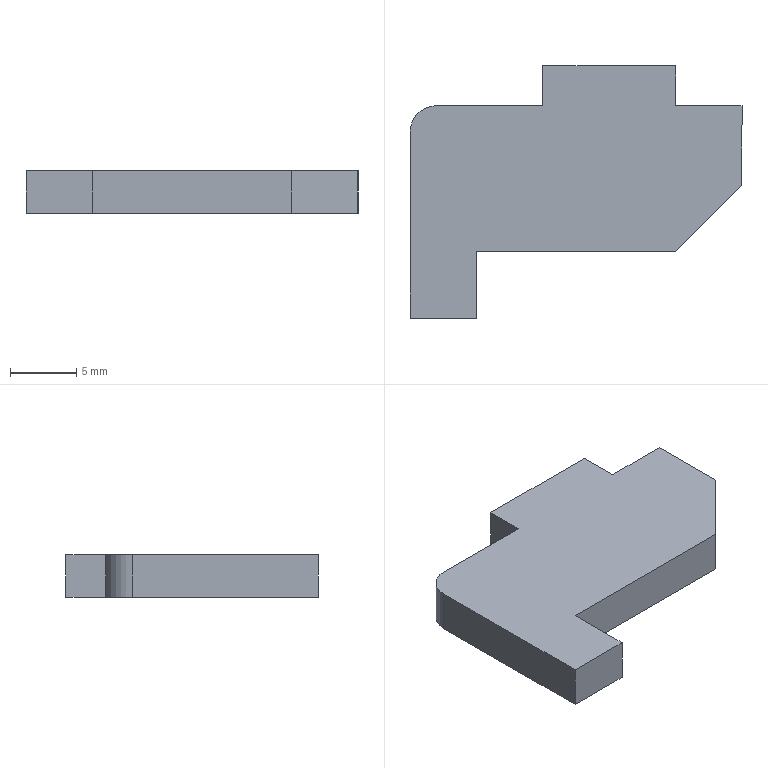Part | SolidWorks | features FlatPattern 1, SMBaseFlange 1, SheetMetal 1 | 1 solid | 14 faces | box 25 x 19 x 3.2 mm | volume 1013 mm3 | plane 13 | cylinder 1 | commonest cylinder face diameters 4 x1
STEP:
#1=CARTESIAN_POINT('',(-81.748,-105.118,0.));
#2=VERTEX_POINT('',#1);
#3=CARTESIAN_POINT('',(-81.748,-100.118,0.));
#4=VERTEX_POINT('',#3);
#5=CARTESIAN_POINT('',(-81.748,-100.118,0.));
#6=DIRECTION('',(0.,1.,0.));
#7=VECTOR('',#6,1000.);
#8=LINE('',#5,#7);
#9=EDGE_CURVE('',#2,#4,#8,.T.);
#10=ORIENTED_EDGE('',*,*,#9,.F.);
#11=CARTESIAN_POINT('',(-81.748,-105.118,-3.2));
#12=VERTEX_POINT('',#11);
#13=CARTESIAN_POINT('',(-81.748,-105.118,-3.2));
#14=DIRECTION('',(0.,0.,1.));
#15=VECTOR('',#14,1000.);
#16=LINE('',#13,#15);
#17=EDGE_CURVE('',#12,#2,#16,.T.);
#18=ORIENTED_EDGE('',*,*,#17,.F.);
#19=CARTESIAN_POINT('',(-81.748,-100.118,-3.2));
#20=VERTEX_POINT('',#19);
#21=CARTESIAN_POINT('',(-81.748,-100.118,-3.2));
#22=DIRECTION('',(0.,1.,0.));
#23=VECTOR('',#22,1000.);
#24=LINE('',#21,#23);
#25=EDGE_CURVE('',#12,#20,#24,.T.);
#26=ORIENTED_EDGE('',*,*,#25,.T.);
#27=CARTESIAN_POINT('',(-81.748,-100.118,-3.2));
#28=DIRECTION('',(0.,0.,1.));
#29=VECTOR('',#28,1000.);
#30=LINE('',#27,#29);
#31=EDGE_CURVE('',#20,#4,#30,.T.);
#32=ORIENTED_EDGE('',*,*,#31,.T.);
#33=EDGE_LOOP('',(#10,#18,#26,#32));
#34=FACE_OUTER_BOUND('',#33,.T.);
#35=CARTESIAN_POINT('',(-81.748,-100.118,-3.2));
#36=DIRECTION('',(1.,0.,0.));
#37=DIRECTION('',(0.,0.,-1.));
#38=AXIS2_PLACEMENT_3D('',#35,#36,#37);
#39=PLANE('',#38);
#40=ADVANCED_FACE('',(#34),#39,.T.);
#41=CARTESIAN_POINT('',(-86.748,-105.118,0.));
#42=VERTEX_POINT('',#41);
#43=CARTESIAN_POINT('',(-81.748,-105.118,0.));
#44=DIRECTION('',(1.,0.,0.));
#45=VECTOR('',#44,1000.);
#46=LINE('',#43,#45);
#47=EDGE_CURVE('',#42,#2,#46,.T.);
#48=ORIENTED_EDGE('',*,*,#47,.F.);
#49=CARTESIAN_POINT('',(-86.748,-105.118,-3.2));
#50=VERTEX_POINT('',#49);
#51=CARTESIAN_POINT('',(-86.748,-105.118,-3.2));
#52=DIRECTION('',(0.,0.,1.));
#53=VECTOR('',#52,1000.);
#54=LINE('',#51,#53);
#55=EDGE_CURVE('',#50,#42,#54,.T.);
#56=ORIENTED_EDGE('',*,*,#55,.F.);
#57=CARTESIAN_POINT('',(-81.748,-105.118,-3.2));
#58=DIRECTION('',(1.,0.,0.));
#59=VECTOR('',#58,1000.);
#60=LINE('',#57,#59);
#61=EDGE_CURVE('',#50,#12,#60,.T.);
#62=ORIENTED_EDGE('',*,*,#61,.T.);
#63=ORIENTED_EDGE('',*,*,#17,.T.);
#64=EDGE_LOOP('',(#48,#56,#62,#63));
#65=FACE_OUTER_BOUND('',#64,.T.);
#66=CARTESIAN_POINT('',(-81.748,-105.118,-3.2));
#67=DIRECTION('',(0.,-1.,0.));
#68=DIRECTION('',(0.,0.,-1.));
#69=AXIS2_PLACEMENT_3D('',#66,#67,#68);
#70=PLANE('',#69);
#71=ADVANCED_FACE('',(#65),#70,.T.);
#72=CARTESIAN_POINT('',(-86.748,-91.118,0.));
#73=VERTEX_POINT('',#72);
#74=CARTESIAN_POINT('',(-86.748,-105.118,0.));
#75=DIRECTION('',(0.,-1.,0.));
#76=VECTOR('',#75,1000.);
#77=LINE('',#74,#76);
#78=EDGE_CURVE('',#73,#42,#77,.T.);
#79=ORIENTED_EDGE('',*,*,#78,.F.);
#80=CARTESIAN_POINT('',(-86.748,-91.118,-3.2));
#81=VERTEX_POINT('',#80);
#82=CARTESIAN_POINT('',(-86.748,-91.118,-3.2));
#83=DIRECTION('',(0.,0.,1.));
#84=VECTOR('',#83,1000.);
#85=LINE('',#82,#84);
#86=EDGE_CURVE('',#81,#73,#85,.T.);
#87=ORIENTED_EDGE('',*,*,#86,.F.);
#88=CARTESIAN_POINT('',(-86.748,-105.118,-3.2));
#89=DIRECTION('',(0.,-1.,0.));
#90=VECTOR('',#89,1000.);
#91=LINE('',#88,#90);
#92=EDGE_CURVE('',#81,#50,#91,.T.);
#93=ORIENTED_EDGE('',*,*,#92,.T.);
#94=ORIENTED_EDGE('',*,*,#55,.T.);
#95=EDGE_LOOP('',(#79,#87,#93,#94));
#96=FACE_OUTER_BOUND('',#95,.T.);
#97=CARTESIAN_POINT('',(-86.748,-105.118,-3.2));
#98=DIRECTION('',(-1.,0.,0.));
#99=DIRECTION('',(0.,0.,1.));
#100=AXIS2_PLACEMENT_3D('',#97,#98,#99);
#101=PLANE('',#100);
#102=ADVANCED_FACE('',(#96),#101,.T.);
#103=CARTESIAN_POINT('',(-84.748,-89.118,0.));
#104=VERTEX_POINT('',#103);
#105=CARTESIAN_POINT('',(-84.748,-91.118,0.));
#106=DIRECTION('',(0.,0.,1.));
#107=DIRECTION('',(-1.,0.,0.));
#108=AXIS2_PLACEMENT_3D('',#105,#106,#107);
#109=CIRCLE('',#108,2.);
#110=EDGE_CURVE('',#104,#73,#109,.T.);
#111=ORIENTED_EDGE('',*,*,#110,.F.);
#112=CARTESIAN_POINT('',(-84.748,-89.118,-3.2));
#113=VERTEX_POINT('',#112);
#114=CARTESIAN_POINT('',(-84.748,-89.118,-3.2));
#115=DIRECTION('',(0.,0.,1.));
#116=VECTOR('',#115,1000.);
#117=LINE('',#114,#116);
#118=EDGE_CURVE('',#113,#104,#117,.T.);
#119=ORIENTED_EDGE('',*,*,#118,.F.);
#120=CARTESIAN_POINT('',(-84.748,-91.118,-3.2));
#121=DIRECTION('',(0.,0.,1.));
#122=DIRECTION('',(-1.,0.,0.));
#123=AXIS2_PLACEMENT_3D('',#120,#121,#122);
#124=CIRCLE('',#123,2.);
#125=EDGE_CURVE('',#113,#81,#124,.T.);
#126=ORIENTED_EDGE('',*,*,#125,.T.);
#127=ORIENTED_EDGE('',*,*,#86,.T.);
#128=EDGE_LOOP('',(#111,#119,#126,#127));
#129=FACE_OUTER_BOUND('',#128,.T.);
#130=CARTESIAN_POINT('',(-84.748,-91.118,-3.2));
#131=DIRECTION('',(0.,0.,1.));
#132=DIRECTION('',(1.,0.,0.));
#133=AXIS2_PLACEMENT_3D('',#130,#131,#132);
#134=CYLINDRICAL_SURFACE('',#133,2.);
#135=ADVANCED_FACE('',(#129),#134,.T.);
#136=CARTESIAN_POINT('',(-76.748,-89.118,0.));
#137=VERTEX_POINT('',#136);
#138=CARTESIAN_POINT('',(-84.748,-89.118,0.));
#139=DIRECTION('',(-1.,0.,0.));
#140=VECTOR('',#139,1000.);
#141=LINE('',#138,#140);
#142=EDGE_CURVE('',#137,#104,#141,.T.);
#143=ORIENTED_EDGE('',*,*,#142,.F.);
#144=CARTESIAN_POINT('',(-76.748,-89.118,-3.2));
#145=VERTEX_POINT('',#144);
#146=CARTESIAN_POINT('',(-76.748,-89.118,-3.2));
#147=DIRECTION('',(0.,0.,1.));
#148=VECTOR('',#147,1000.);
#149=LINE('',#146,#148);
#150=EDGE_CURVE('',#145,#137,#149,.T.);
#151=ORIENTED_EDGE('',*,*,#150,.F.);
#152=CARTESIAN_POINT('',(-84.748,-89.118,-3.2));
#153=DIRECTION('',(-1.,0.,0.));
#154=VECTOR('',#153,1000.);
#155=LINE('',#152,#154);
#156=EDGE_CURVE('',#145,#113,#155,.T.);
#157=ORIENTED_EDGE('',*,*,#156,.T.);
#158=ORIENTED_EDGE('',*,*,#118,.T.);
#159=EDGE_LOOP('',(#143,#151,#157,#158));
#160=FACE_OUTER_BOUND('',#159,.T.);
#161=CARTESIAN_POINT('',(-84.748,-89.118,-3.2));
#162=DIRECTION('',(0.,1.,0.));
#163=DIRECTION('',(0.,0.,1.));
#164=AXIS2_PLACEMENT_3D('',#161,#162,#163);
#165=PLANE('',#164);
#166=ADVANCED_FACE('',(#160),#165,.T.);
#167=CARTESIAN_POINT('',(-76.748,-86.118,0.));
#168=VERTEX_POINT('',#167);
#169=CARTESIAN_POINT('',(-76.748,-89.118,0.));
#170=DIRECTION('',(0.,-1.,0.));
#171=VECTOR('',#170,1000.);
#172=LINE('',#169,#171);
#173=EDGE_CURVE('',#168,#137,#172,.T.);
#174=ORIENTED_EDGE('',*,*,#173,.F.);
#175=CARTESIAN_POINT('',(-76.748,-86.118,-3.2));
#176=VERTEX_POINT('',#175);
#177=CARTESIAN_POINT('',(-76.748,-86.118,-3.2));
#178=DIRECTION('',(0.,0.,1.));
#179=VECTOR('',#178,1000.);
#180=LINE('',#177,#179);
#181=EDGE_CURVE('',#176,#168,#180,.T.);
#182=ORIENTED_EDGE('',*,*,#181,.F.);
#183=CARTESIAN_POINT('',(-76.748,-89.118,-3.2));
#184=DIRECTION('',(0.,-1.,0.));
#185=VECTOR('',#184,1000.);
#186=LINE('',#183,#185);
#187=EDGE_CURVE('',#176,#145,#186,.T.);
#188=ORIENTED_EDGE('',*,*,#187,.T.);
#189=ORIENTED_EDGE('',*,*,#150,.T.);
#190=EDGE_LOOP('',(#174,#182,#188,#189));
#191=FACE_OUTER_BOUND('',#190,.T.);
#192=CARTESIAN_POINT('',(-76.748,-89.118,-3.2));
#193=DIRECTION('',(-1.,0.,0.));
#194=DIRECTION('',(0.,0.,1.));
#195=AXIS2_PLACEMENT_3D('',#192,#193,#194);
#196=PLANE('',#195);
#197=ADVANCED_FACE('',(#191),#196,.T.);
#198=CARTESIAN_POINT('',(-66.748,-86.118,0.));
#199=VERTEX_POINT('',#198);
#200=CARTESIAN_POINT('',(-76.748,-86.118,0.));
#201=DIRECTION('',(-1.,0.,0.));
#202=VECTOR('',#201,1000.);
#203=LINE('',#200,#202);
#204=EDGE_CURVE('',#199,#168,#203,.T.);
#205=ORIENTED_EDGE('',*,*,#204,.F.);
#206=CARTESIAN_POINT('',(-66.748,-86.118,-3.2));
#207=VERTEX_POINT('',#206);
#208=CARTESIAN_POINT('',(-66.748,-86.118,-3.2));
#209=DIRECTION('',(0.,0.,1.));
#210=VECTOR('',#209,1000.);
#211=LINE('',#208,#210);
#212=EDGE_CURVE('',#207,#199,#211,.T.);
#213=ORIENTED_EDGE('',*,*,#212,.F.);
#214=CARTESIAN_POINT('',(-76.748,-86.118,-3.2));
#215=DIRECTION('',(-1.,0.,0.));
#216=VECTOR('',#215,1000.);
#217=LINE('',#214,#216);
#218=EDGE_CURVE('',#207,#176,#217,.T.);
#219=ORIENTED_EDGE('',*,*,#218,.T.);
#220=ORIENTED_EDGE('',*,*,#181,.T.);
#221=EDGE_LOOP('',(#205,#213,#219,#220));
#222=FACE_OUTER_BOUND('',#221,.T.);
#223=CARTESIAN_POINT('',(-76.748,-86.118,-3.2));
#224=DIRECTION('',(0.,1.,0.));
#225=DIRECTION('',(0.,0.,1.));
#226=AXIS2_PLACEMENT_3D('',#223,#224,#225);
#227=PLANE('',#226);
#228=ADVANCED_FACE('',(#222),#227,.T.);
#229=CARTESIAN_POINT('',(-66.748,-89.118,0.));
#230=VERTEX_POINT('',#229);
#231=CARTESIAN_POINT('',(-66.748,-86.118,0.));
#232=DIRECTION('',(0.,1.,0.));
#233=VECTOR('',#232,1000.);
#234=LINE('',#231,#233);
#235=EDGE_CURVE('',#230,#199,#234,.T.);
#236=ORIENTED_EDGE('',*,*,#235,.F.);
#237=CARTESIAN_POINT('',(-66.748,-89.118,-3.2));
#238=VERTEX_POINT('',#237);
#239=CARTESIAN_POINT('',(-66.748,-89.118,-3.2));
#240=DIRECTION('',(0.,0.,1.));
#241=VECTOR('',#240,1000.);
#242=LINE('',#239,#241);
#243=EDGE_CURVE('',#238,#230,#242,.T.);
#244=ORIENTED_EDGE('',*,*,#243,.F.);
#245=CARTESIAN_POINT('',(-66.748,-86.118,-3.2));
#246=DIRECTION('',(0.,1.,0.));
#247=VECTOR('',#246,1000.);
#248=LINE('',#245,#247);
#249=EDGE_CURVE('',#238,#207,#248,.T.);
#250=ORIENTED_EDGE('',*,*,#249,.T.);
#251=ORIENTED_EDGE('',*,*,#212,.T.);
#252=EDGE_LOOP('',(#236,#244,#250,#251));
#253=FACE_OUTER_BOUND('',#252,.T.);
#254=CARTESIAN_POINT('',(-66.748,-86.118,-3.2));
#255=DIRECTION('',(1.,0.,0.));
#256=DIRECTION('',(0.,0.,-1.));
#257=AXIS2_PLACEMENT_3D('',#254,#255,#256);
#258=PLANE('',#257);
#259=ADVANCED_FACE('',(#253),#258,.T.);
#260=CARTESIAN_POINT('',(-61.748,-89.118,0.));
#261=VERTEX_POINT('',#260);
#262=CARTESIAN_POINT('',(-66.748,-89.118,0.));
#263=DIRECTION('',(-1.,0.,0.));
#264=VECTOR('',#263,1000.);
#265=LINE('',#262,#264);
#266=EDGE_CURVE('',#261,#230,#265,.T.);
#267=ORIENTED_EDGE('',*,*,#266,.F.);
#268=CARTESIAN_POINT('',(-61.748,-89.118,-3.2));
#269=VERTEX_POINT('',#268);
#270=CARTESIAN_POINT('',(-61.748,-89.118,-3.2));
#271=DIRECTION('',(0.,0.,1.));
#272=VECTOR('',#271,1000.);
#273=LINE('',#270,#272);
#274=EDGE_CURVE('',#269,#261,#273,.T.);
#275=ORIENTED_EDGE('',*,*,#274,.F.);
#276=CARTESIAN_POINT('',(-66.748,-89.118,-3.2));
#277=DIRECTION('',(-1.,0.,0.));
#278=VECTOR('',#277,1000.);
#279=LINE('',#276,#278);
#280=EDGE_CURVE('',#269,#238,#279,.T.);
#281=ORIENTED_EDGE('',*,*,#280,.T.);
#282=ORIENTED_EDGE('',*,*,#243,.T.);
#283=EDGE_LOOP('',(#267,#275,#281,#282));
#284=FACE_OUTER_BOUND('',#283,.T.);
#285=CARTESIAN_POINT('',(-66.748,-89.118,-3.2));
#286=DIRECTION('',(0.,1.,0.));
#287=DIRECTION('',(0.,0.,1.));
#288=AXIS2_PLACEMENT_3D('',#285,#286,#287);
#289=PLANE('',#288);
#290=ADVANCED_FACE('',(#284),#289,.T.);
#291=CARTESIAN_POINT('',(-61.748,-95.118,0.));
#292=VERTEX_POINT('',#291);
#293=CARTESIAN_POINT('',(-61.748,-89.118,0.));
#294=DIRECTION('',(0.,1.,0.));
#295=VECTOR('',#294,1000.);
#296=LINE('',#293,#295);
#297=EDGE_CURVE('',#292,#261,#296,.T.);
#298=ORIENTED_EDGE('',*,*,#297,.F.);
#299=CARTESIAN_POINT('',(-61.748,-95.118,-3.2));
#300=VERTEX_POINT('',#299);
#301=CARTESIAN_POINT('',(-61.748,-95.118,-3.2));
#302=DIRECTION('',(0.,0.,1.));
#303=VECTOR('',#302,1000.);
#304=LINE('',#301,#303);
#305=EDGE_CURVE('',#300,#292,#304,.T.);
#306=ORIENTED_EDGE('',*,*,#305,.F.);
#307=CARTESIAN_POINT('',(-61.748,-89.118,-3.2));
#308=DIRECTION('',(0.,1.,0.));
#309=VECTOR('',#308,1000.);
#310=LINE('',#307,#309);
#311=EDGE_CURVE('',#300,#269,#310,.T.);
#312=ORIENTED_EDGE('',*,*,#311,.T.);
#313=ORIENTED_EDGE('',*,*,#274,.T.);
#314=EDGE_LOOP('',(#298,#306,#312,#313));
#315=FACE_OUTER_BOUND('',#314,.T.);
#316=CARTESIAN_POINT('',(-61.748,-89.118,-3.2));
#317=DIRECTION('',(1.,0.,0.));
#318=DIRECTION('',(0.,1.,0.));
#319=AXIS2_PLACEMENT_3D('',#316,#317,#318);
#320=PLANE('',#319);
#321=ADVANCED_FACE('',(#315),#320,.T.);
#322=CARTESIAN_POINT('',(-66.748,-100.118,0.));
#323=VERTEX_POINT('',#322);
#324=CARTESIAN_POINT('',(-61.748,-95.118,0.));
#325=DIRECTION('',(0.7071,0.7071,0.));
#326=VECTOR('',#325,1000.);
#327=LINE('',#324,#326);
#328=EDGE_CURVE('',#323,#292,#327,.T.);
#329=ORIENTED_EDGE('',*,*,#328,.F.);
#330=CARTESIAN_POINT('',(-66.748,-100.118,-3.2));
#331=VERTEX_POINT('',#330);
#332=CARTESIAN_POINT('',(-66.748,-100.118,-3.2));
#333=DIRECTION('',(0.,0.,1.));
#334=VECTOR('',#333,1000.);
#335=LINE('',#332,#334);
#336=EDGE_CURVE('',#331,#323,#335,.T.);
#337=ORIENTED_EDGE('',*,*,#336,.F.);
#338=CARTESIAN_POINT('',(-61.748,-95.118,-3.2));
#339=DIRECTION('',(0.7071,0.7071,0.));
#340=VECTOR('',#339,1000.);
#341=LINE('',#338,#340);
#342=EDGE_CURVE('',#331,#300,#341,.T.);
#343=ORIENTED_EDGE('',*,*,#342,.T.);
#344=ORIENTED_EDGE('',*,*,#305,.T.);
#345=EDGE_LOOP('',(#329,#337,#343,#344));
#346=FACE_OUTER_BOUND('',#345,.T.);
#347=CARTESIAN_POINT('',(-61.748,-95.118,-3.2));
#348=DIRECTION('',(0.7071,-0.7071,0.));
#349=DIRECTION('',(0.7071,0.7071,0.));
#350=AXIS2_PLACEMENT_3D('',#347,#348,#349);
#351=PLANE('',#350);
#352=ADVANCED_FACE('',(#346),#351,.T.);
#353=CARTESIAN_POINT('',(-66.748,-100.118,0.));
#354=DIRECTION('',(1.,0.,0.));
#355=VECTOR('',#354,1000.);
#356=LINE('',#353,#355);
#357=EDGE_CURVE('',#4,#323,#356,.T.);
#358=ORIENTED_EDGE('',*,*,#357,.F.);
#359=ORIENTED_EDGE('',*,*,#31,.F.);
#360=CARTESIAN_POINT('',(-66.748,-100.118,-3.2));
#361=DIRECTION('',(1.,0.,0.));
#362=VECTOR('',#361,1000.);
#363=LINE('',#360,#362);
#364=EDGE_CURVE('',#20,#331,#363,.T.);
#365=ORIENTED_EDGE('',*,*,#364,.T.);
#366=ORIENTED_EDGE('',*,*,#336,.T.);
#367=EDGE_LOOP('',(#358,#359,#365,#366));
#368=FACE_OUTER_BOUND('',#367,.T.);
#369=CARTESIAN_POINT('',(-66.748,-100.118,-3.2));
#370=DIRECTION('',(0.,-1.,0.));
#371=DIRECTION('',(0.,0.,-1.));
#372=AXIS2_PLACEMENT_3D('',#369,#370,#371);
#373=PLANE('',#372);
#374=ADVANCED_FACE('',(#368),#373,.T.);
#375=ORIENTED_EDGE('',*,*,#25,.F.);
#376=ORIENTED_EDGE('',*,*,#61,.F.);
#377=ORIENTED_EDGE('',*,*,#92,.F.);
#378=ORIENTED_EDGE('',*,*,#125,.F.);
#379=ORIENTED_EDGE('',*,*,#156,.F.);
#380=ORIENTED_EDGE('',*,*,#187,.F.);
#381=ORIENTED_EDGE('',*,*,#218,.F.);
#382=ORIENTED_EDGE('',*,*,#249,.F.);
#383=ORIENTED_EDGE('',*,*,#280,.F.);
#384=ORIENTED_EDGE('',*,*,#311,.F.);
#385=ORIENTED_EDGE('',*,*,#342,.F.);
#386=ORIENTED_EDGE('',*,*,#364,.F.);
#387=EDGE_LOOP('',(#375,#376,#377,#378,#379,#380,#381,#382,#383,#384,#385,#386));
#388=FACE_OUTER_BOUND('',#387,.T.);
#389=CARTESIAN_POINT('',(-84.748,-91.118,-3.2));
#390=DIRECTION('',(0.,0.,-1.));
#391=DIRECTION('',(-1.,0.,0.));
#392=AXIS2_PLACEMENT_3D('',#389,#390,#391);
#393=PLANE('',#392);
#394=ADVANCED_FACE('',(#388),#393,.T.);
#395=ORIENTED_EDGE('',*,*,#9,.T.);
#396=ORIENTED_EDGE('',*,*,#357,.T.);
#397=ORIENTED_EDGE('',*,*,#328,.T.);
#398=ORIENTED_EDGE('',*,*,#297,.T.);
#399=ORIENTED_EDGE('',*,*,#266,.T.);
#400=ORIENTED_EDGE('',*,*,#235,.T.);
#401=ORIENTED_EDGE('',*,*,#204,.T.);
#402=ORIENTED_EDGE('',*,*,#173,.T.);
#403=ORIENTED_EDGE('',*,*,#142,.T.);
#404=ORIENTED_EDGE('',*,*,#110,.T.);
#405=ORIENTED_EDGE('',*,*,#78,.T.);
#406=ORIENTED_EDGE('',*,*,#47,.T.);
#407=EDGE_LOOP('',(#395,#396,#397,#398,#399,#400,#401,#402,#403,#404,#405,#406));
#408=FACE_OUTER_BOUND('',#407,.T.);
#409=CARTESIAN_POINT('',(-84.748,-91.118,0.));
#410=DIRECTION('',(0.,0.,-1.));
#411=DIRECTION('',(-1.,0.,0.));
#412=AXIS2_PLACEMENT_3D('',#409,#410,#411);
#413=PLANE('',#412);
#414=ADVANCED_FACE('',(#408),#413,.F.);
#415=CLOSED_SHELL('',(#40,#71,#102,#135,#166,#197,#228,#259,#290,#321,#352,#374,#394,#414));
#416=MANIFOLD_SOLID_BREP('',#415);
#417=CARTESIAN_POINT('',(0.,0.,0.));
#418=DIRECTION('',(0.,0.,1.));
#419=DIRECTION('',(1.,0.,0.));
#420=AXIS2_PLACEMENT_3D('',#417,#418,#419);
#421=(LENGTH_UNIT()NAMED_UNIT(*)SI_UNIT(.MILLI.,.METRE.));
#422=UNCERTAINTY_MEASURE_WITH_UNIT(LENGTH_MEASURE(0.00001),#421,'','');
#423=(NAMED_UNIT(*)PLANE_ANGLE_UNIT()SI_UNIT($,.RADIAN.));
#424=(NAMED_UNIT(*)SI_UNIT($,.STERADIAN.)SOLID_ANGLE_UNIT());
#425=(GEOMETRIC_REPRESENTATION_CONTEXT(3)GLOBAL_UNCERTAINTY_ASSIGNED_CONTEXT((#422))GLOBAL_UNIT_ASSIGNED_CONTEXT((#421,#423,#424))REPRESENTATION_CONTEXT('',''));
#426=ADVANCED_BREP_SHAPE_REPRESENTATION('',(#416,#420),#425);